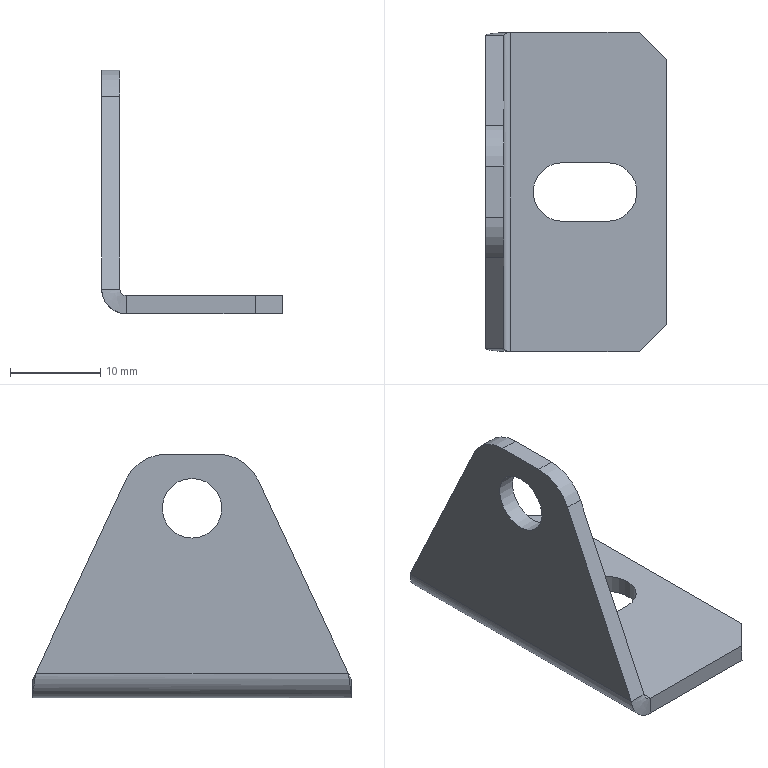Part | NX | 1 solid | 23 faces | box 20 x 35.337 x 27 mm | volume 2319 mm3 | plane 14 | cylinder 7 | spline 2 | commonest cylinder face diameters 6.5 x2 10 x2 1.473 x1 5.473 x1 6.6 x1
STEP:
#1=CARTESIAN_POINT('',(-2.5,3.25,-2.));
#2=VERTEX_POINT('',#1);
#3=CARTESIAN_POINT('',(-2.5,-3.25,-2.));
#4=VERTEX_POINT('',#3);
#5=CARTESIAN_POINT('',(-2.5,0.,-2.));
#6=DIRECTION('',(0.,0.,1.));
#7=DIRECTION('',(1.,0.,0.));
#8=AXIS2_PLACEMENT_3D('',#5,#6,#7);
#9=CIRCLE('',#8,3.25);
#10=EDGE_CURVE('',#2,#4,#9,.T.);
#11=ORIENTED_EDGE('',*,*,#10,.T.);
#12=CARTESIAN_POINT('',(2.5,-3.25,-2.));
#13=VERTEX_POINT('',#12);
#14=CARTESIAN_POINT('',(-2.5,-3.25,-2.));
#15=DIRECTION('',(1.,0.,0.));
#16=VECTOR('',#15,1000.);
#17=LINE('',#14,#16);
#18=EDGE_CURVE('',#4,#13,#17,.T.);
#19=ORIENTED_EDGE('',*,*,#18,.T.);
#20=CARTESIAN_POINT('',(2.5,3.25,-2.));
#21=VERTEX_POINT('',#20);
#22=CARTESIAN_POINT('',(2.5,0.,-2.));
#23=DIRECTION('',(0.,0.,1.));
#24=DIRECTION('',(1.,0.,0.));
#25=AXIS2_PLACEMENT_3D('',#22,#23,#24);
#26=CIRCLE('',#25,3.25);
#27=EDGE_CURVE('',#13,#21,#26,.T.);
#28=ORIENTED_EDGE('',*,*,#27,.T.);
#29=CARTESIAN_POINT('',(-2.5,3.25,-2.));
#30=DIRECTION('',(-1.,0.,0.));
#31=VECTOR('',#30,1000.);
#32=LINE('',#29,#31);
#33=EDGE_CURVE('',#21,#2,#32,.T.);
#34=ORIENTED_EDGE('',*,*,#33,.T.);
#35=EDGE_LOOP('',(#11,#19,#28,#34));
#36=FACE_BOUND('',#35,.T.);
#37=CARTESIAN_POINT('',(9.,-14.667,-2.));
#38=VERTEX_POINT('',#37);
#39=CARTESIAN_POINT('',(9.,14.67,-2.));
#40=VERTEX_POINT('',#39);
#41=CARTESIAN_POINT('',(9.,-20.,-2.));
#42=DIRECTION('',(0.,1.,0.));
#43=VECTOR('',#42,1000.);
#44=LINE('',#41,#43);
#45=EDGE_CURVE('',#38,#40,#44,.T.);
#46=ORIENTED_EDGE('',*,*,#45,.F.);
#47=CARTESIAN_POINT('',(6.,-17.667,-2.));
#48=VERTEX_POINT('',#47);
#49=CARTESIAN_POINT('',(11.833,-11.833,-2.));
#50=DIRECTION('',(0.7071,0.7071,0.));
#51=VECTOR('',#50,1000.);
#52=LINE('',#49,#51);
#53=EDGE_CURVE('',#38,#48,#52,.F.);
#54=ORIENTED_EDGE('',*,*,#53,.T.);
#55=CARTESIAN_POINT('',(-8.263,-17.667,-2.));
#56=VERTEX_POINT('',#55);
#57=CARTESIAN_POINT('',(0.,-17.667,-2.));
#58=DIRECTION('',(-1.,0.,0.));
#59=VECTOR('',#58,1000.);
#60=LINE('',#57,#59);
#61=EDGE_CURVE('',#48,#56,#60,.T.);
#62=ORIENTED_EDGE('',*,*,#61,.T.);
#63=CARTESIAN_POINT('',(-8.263,17.67,-2.));
#64=VERTEX_POINT('',#63);
#65=CARTESIAN_POINT('',(-8.263,-20.,-2.));
#66=DIRECTION('',(0.,-1.,0.));
#67=VECTOR('',#66,1000.);
#68=LINE('',#65,#67);
#69=EDGE_CURVE('',#56,#64,#68,.F.);
#70=ORIENTED_EDGE('',*,*,#69,.T.);
#71=CARTESIAN_POINT('',(6.,17.67,-2.));
#72=VERTEX_POINT('',#71);
#73=CARTESIAN_POINT('',(0.,17.67,-2.));
#74=DIRECTION('',(-1.,0.,0.));
#75=VECTOR('',#74,1000.);
#76=LINE('',#73,#75);
#77=EDGE_CURVE('',#64,#72,#76,.F.);
#78=ORIENTED_EDGE('',*,*,#77,.T.);
#79=CARTESIAN_POINT('',(11.835,11.835,-2.));
#80=DIRECTION('',(-0.7071,0.7071,0.));
#81=VECTOR('',#80,1000.);
#82=LINE('',#79,#81);
#83=EDGE_CURVE('',#72,#40,#82,.F.);
#84=ORIENTED_EDGE('',*,*,#83,.T.);
#85=EDGE_LOOP('',(#46,#54,#62,#70,#78,#84));
#86=FACE_BOUND('',#85,.T.);
#87=CARTESIAN_POINT('',(0.,0.,-2.));
#88=DIRECTION('',(0.,0.,-1.));
#89=DIRECTION('',(-1.,0.,0.));
#90=AXIS2_PLACEMENT_3D('',#87,#88,#89);
#91=PLANE('',#90);
#92=ADVANCED_FACE('',(#36,#86),#91,.T.);
#93=CARTESIAN_POINT('',(-2.5,-3.25,0.));
#94=VERTEX_POINT('',#93);
#95=CARTESIAN_POINT('',(2.5,-3.25,0.));
#96=VERTEX_POINT('',#95);
#97=CARTESIAN_POINT('',(-2.5,-3.25,0.));
#98=DIRECTION('',(1.,0.,0.));
#99=VECTOR('',#98,1000.);
#100=LINE('',#97,#99);
#101=EDGE_CURVE('',#94,#96,#100,.T.);
#102=ORIENTED_EDGE('',*,*,#101,.F.);
#103=CARTESIAN_POINT('',(-2.5,3.25,0.));
#104=VERTEX_POINT('',#103);
#105=CARTESIAN_POINT('',(-2.5,0.,0.));
#106=DIRECTION('',(0.,0.,1.));
#107=DIRECTION('',(1.,0.,0.));
#108=AXIS2_PLACEMENT_3D('',#105,#106,#107);
#109=CIRCLE('',#108,3.25);
#110=EDGE_CURVE('',#104,#94,#109,.T.);
#111=ORIENTED_EDGE('',*,*,#110,.F.);
#112=CARTESIAN_POINT('',(2.5,3.25,0.));
#113=VERTEX_POINT('',#112);
#114=CARTESIAN_POINT('',(-2.5,3.25,0.));
#115=DIRECTION('',(-1.,0.,0.));
#116=VECTOR('',#115,1000.);
#117=LINE('',#114,#116);
#118=EDGE_CURVE('',#113,#104,#117,.T.);
#119=ORIENTED_EDGE('',*,*,#118,.F.);
#120=CARTESIAN_POINT('',(2.5,0.,0.));
#121=DIRECTION('',(0.,0.,1.));
#122=DIRECTION('',(1.,0.,0.));
#123=AXIS2_PLACEMENT_3D('',#120,#121,#122);
#124=CIRCLE('',#123,3.25);
#125=EDGE_CURVE('',#96,#113,#124,.T.);
#126=ORIENTED_EDGE('',*,*,#125,.F.);
#127=EDGE_LOOP('',(#102,#111,#119,#126));
#128=FACE_BOUND('',#127,.T.);
#129=CARTESIAN_POINT('',(6.,-17.667,0.));
#130=VERTEX_POINT('',#129);
#131=CARTESIAN_POINT('',(-8.263,-17.667,0.));
#132=VERTEX_POINT('',#131);
#133=CARTESIAN_POINT('',(0.,-17.667,0.));
#134=DIRECTION('',(-1.,0.,0.));
#135=VECTOR('',#134,1000.);
#136=LINE('',#133,#135);
#137=EDGE_CURVE('',#130,#132,#136,.T.);
#138=ORIENTED_EDGE('',*,*,#137,.F.);
#139=CARTESIAN_POINT('',(9.,-14.667,0.));
#140=VERTEX_POINT('',#139);
#141=CARTESIAN_POINT('',(9.,-14.667,0.));
#142=DIRECTION('',(-0.7071,-0.7071,0.));
#143=VECTOR('',#142,1000.);
#144=LINE('',#141,#143);
#145=EDGE_CURVE('',#130,#140,#144,.F.);
#146=ORIENTED_EDGE('',*,*,#145,.T.);
#147=CARTESIAN_POINT('',(9.,14.67,0.));
#148=VERTEX_POINT('',#147);
#149=CARTESIAN_POINT('',(9.,-20.,0.));
#150=DIRECTION('',(0.,1.,0.));
#151=VECTOR('',#150,1000.);
#152=LINE('',#149,#151);
#153=EDGE_CURVE('',#140,#148,#152,.T.);
#154=ORIENTED_EDGE('',*,*,#153,.T.);
#155=CARTESIAN_POINT('',(6.,17.67,0.));
#156=VERTEX_POINT('',#155);
#157=CARTESIAN_POINT('',(6.,17.67,0.));
#158=DIRECTION('',(0.7071,-0.7071,0.));
#159=VECTOR('',#158,1000.);
#160=LINE('',#157,#159);
#161=EDGE_CURVE('',#148,#156,#160,.F.);
#162=ORIENTED_EDGE('',*,*,#161,.T.);
#163=CARTESIAN_POINT('',(-8.263,17.67,0.));
#164=VERTEX_POINT('',#163);
#165=CARTESIAN_POINT('',(0.,17.67,0.));
#166=DIRECTION('',(1.,0.,0.));
#167=VECTOR('',#166,1000.);
#168=LINE('',#165,#167);
#169=EDGE_CURVE('',#164,#156,#168,.T.);
#170=ORIENTED_EDGE('',*,*,#169,.F.);
#171=CARTESIAN_POINT('',(-8.263,-20.,0.));
#172=DIRECTION('',(0.,-1.,0.));
#173=VECTOR('',#172,1000.);
#174=LINE('',#171,#173);
#175=EDGE_CURVE('',#132,#164,#174,.F.);
#176=ORIENTED_EDGE('',*,*,#175,.F.);
#177=EDGE_LOOP('',(#138,#146,#154,#162,#170,#176));
#178=FACE_BOUND('',#177,.T.);
#179=CARTESIAN_POINT('',(0.,0.,0.));
#180=DIRECTION('',(0.,0.,-1.));
#181=DIRECTION('',(-1.,0.,0.));
#182=AXIS2_PLACEMENT_3D('',#179,#180,#181);
#183=PLANE('',#182);
#184=ADVANCED_FACE('',(#128,#178),#183,.F.);
#185=ORIENTED_EDGE('',*,*,#153,.F.);
#186=CARTESIAN_POINT('',(9.,-14.667,-2.));
#187=DIRECTION('',(0.,0.,-1.));
#188=VECTOR('',#187,1000.);
#189=LINE('',#186,#188);
#190=EDGE_CURVE('',#140,#38,#189,.T.);
#191=ORIENTED_EDGE('',*,*,#190,.T.);
#192=ORIENTED_EDGE('',*,*,#45,.T.);
#193=CARTESIAN_POINT('',(9.,14.67,-2.));
#194=DIRECTION('',(0.,0.,1.));
#195=VECTOR('',#194,1000.);
#196=LINE('',#193,#195);
#197=EDGE_CURVE('',#40,#148,#196,.T.);
#198=ORIENTED_EDGE('',*,*,#197,.T.);
#199=EDGE_LOOP('',(#185,#191,#192,#198));
#200=FACE_BOUND('',#199,.T.);
#201=CARTESIAN_POINT('',(9.,-20.,-2.));
#202=DIRECTION('',(1.,0.,0.));
#203=DIRECTION('',(0.,0.,-1.));
#204=AXIS2_PLACEMENT_3D('',#201,#202,#203);
#205=PLANE('',#204);
#206=ADVANCED_FACE('',(#200),#205,.T.);
#207=CARTESIAN_POINT('',(-11.,-17.323,0.7366));
#208=VERTEX_POINT('',#207);
#209=CARTESIAN_POINT('',(-11.,17.327,0.7366));
#210=VERTEX_POINT('',#209);
#211=CARTESIAN_POINT('',(-11.,0.,0.7366));
#212=DIRECTION('',(0.,1.,0.));
#213=VECTOR('',#212,1000.);
#214=LINE('',#211,#213);
#215=EDGE_CURVE('',#208,#210,#214,.T.);
#216=ORIENTED_EDGE('',*,*,#215,.T.);
#217=CARTESIAN_POINT('',(-8.263,17.327,0.7366));
#218=DIRECTION('',(0.,0.9922,0.1244));
#219=DIRECTION('',(0.,-0.1244,0.9922));
#220=AXIS2_PLACEMENT_3D('',#217,#218,#219);
#221=ELLIPSE('',#220,2.758,2.737);
#222=EDGE_CURVE('',#210,#64,#221,.F.);
#223=ORIENTED_EDGE('',*,*,#222,.T.);
#224=ORIENTED_EDGE('',*,*,#69,.F.);
#225=CARTESIAN_POINT('',(-8.263,-17.323,0.7366));
#226=DIRECTION('',(0.,-0.9922,0.1246));
#227=DIRECTION('',(0.,-0.1246,-0.9922));
#228=AXIS2_PLACEMENT_3D('',#225,#226,#227);
#229=ELLIPSE('',#228,2.758,2.737);
#230=EDGE_CURVE('',#56,#208,#229,.F.);
#231=ORIENTED_EDGE('',*,*,#230,.T.);
#232=EDGE_LOOP('',(#216,#223,#224,#231));
#233=FACE_BOUND('',#232,.T.);
#234=CARTESIAN_POINT('',(-8.263,-20.,0.7366));
#235=DIRECTION('',(0.,-1.,0.));
#236=DIRECTION('',(-1.,0.,0.));
#237=AXIS2_PLACEMENT_3D('',#234,#235,#236);
#238=CYLINDRICAL_SURFACE('',#237,2.737);
#239=ADVANCED_FACE('',(#233),#238,.T.);
#240=CARTESIAN_POINT('',(-9.,17.327,0.7366));
#241=VERTEX_POINT('',#240);
#242=CARTESIAN_POINT('',(-8.263,17.327,0.7366));
#243=DIRECTION('',(0.,0.9064,0.4224));
#244=DIRECTION('',(0.,-0.4224,0.9064));
#245=AXIS2_PLACEMENT_3D('',#242,#243,#244);
#246=ELLIPSE('',#245,0.8126,0.7366);
#247=EDGE_CURVE('',#241,#164,#246,.F.);
#248=ORIENTED_EDGE('',*,*,#247,.F.);
#249=CARTESIAN_POINT('',(-9.,-17.323,0.7366));
#250=VERTEX_POINT('',#249);
#251=CARTESIAN_POINT('',(-9.,20.,0.7366));
#252=DIRECTION('',(0.,-1.,0.));
#253=VECTOR('',#252,1000.);
#254=LINE('',#251,#253);
#255=EDGE_CURVE('',#241,#250,#254,.T.);
#256=ORIENTED_EDGE('',*,*,#255,.T.);
#257=CARTESIAN_POINT('',(-8.263,-17.323,0.7366));
#258=DIRECTION('',(0.,-0.9062,0.4229));
#259=DIRECTION('',(0.,-0.4229,-0.9062));
#260=AXIS2_PLACEMENT_3D('',#257,#258,#259);
#261=ELLIPSE('',#260,0.8129,0.7366);
#262=EDGE_CURVE('',#132,#250,#261,.F.);
#263=ORIENTED_EDGE('',*,*,#262,.F.);
#264=ORIENTED_EDGE('',*,*,#175,.T.);
#265=EDGE_LOOP('',(#248,#256,#263,#264));
#266=FACE_BOUND('',#265,.T.);
#267=CARTESIAN_POINT('',(-8.263,-20.,0.7366));
#268=DIRECTION('',(0.,-1.,0.));
#269=DIRECTION('',(-1.,0.,0.));
#270=AXIS2_PLACEMENT_3D('',#267,#268,#269);
#271=CYLINDRICAL_SURFACE('',#270,0.7366);
#272=ADVANCED_FACE('',(#266),#271,.F.);
#273=CARTESIAN_POINT('',(-11.,0.,22.3));
#274=VERTEX_POINT('',#273);
#275=CARTESIAN_POINT('',(-11.,0.,19.));
#276=DIRECTION('',(-1.,0.,0.));
#277=DIRECTION('',(0.,0.,1.));
#278=AXIS2_PLACEMENT_3D('',#275,#276,#277);
#279=CIRCLE('',#278,3.3);
#280=EDGE_CURVE('',#274,#274,#279,.T.);
#281=ORIENTED_EDGE('',*,*,#280,.F.);
#282=EDGE_LOOP('',(#281));
#283=FACE_BOUND('',#282,.T.);
#284=CARTESIAN_POINT('',(-11.,-2.816,25.));
#285=VERTEX_POINT('',#284);
#286=CARTESIAN_POINT('',(-11.,2.835,25.));
#287=VERTEX_POINT('',#286);
#288=CARTESIAN_POINT('',(-11.,20.,25.));
#289=DIRECTION('',(0.,1.,0.));
#290=VECTOR('',#289,1000.);
#291=LINE('',#288,#290);
#292=EDGE_CURVE('',#285,#287,#291,.T.);
#293=ORIENTED_EDGE('',*,*,#292,.T.);
#294=CARTESIAN_POINT('',(-11.,7.367,22.112));
#295=VERTEX_POINT('',#294);
#296=CARTESIAN_POINT('',(-11.,2.835,20.));
#297=DIRECTION('',(1.,0.,0.));
#298=DIRECTION('',(0.,0.,-1.));
#299=AXIS2_PLACEMENT_3D('',#296,#297,#298);
#300=CIRCLE('',#299,5.);
#301=EDGE_CURVE('',#287,#295,#300,.F.);
#302=ORIENTED_EDGE('',*,*,#301,.T.);
#303=CARTESIAN_POINT('',(-11.,14.518,6.765));
#304=DIRECTION('',(0.,-0.4224,0.9064));
#305=VECTOR('',#304,1000.);
#306=LINE('',#303,#305);
#307=EDGE_CURVE('',#210,#295,#306,.T.);
#308=ORIENTED_EDGE('',*,*,#307,.F.);
#309=ORIENTED_EDGE('',*,*,#215,.F.);
#310=CARTESIAN_POINT('',(-11.,-7.347,22.114));
#311=VERTEX_POINT('',#310);
#312=CARTESIAN_POINT('',(-11.,-6.,25.));
#313=DIRECTION('',(0.,0.4229,0.9062));
#314=VECTOR('',#313,1000.);
#315=LINE('',#312,#314);
#316=EDGE_CURVE('',#208,#311,#315,.T.);
#317=ORIENTED_EDGE('',*,*,#316,.T.);
#318=CARTESIAN_POINT('',(-11.,-2.816,20.));
#319=DIRECTION('',(1.,0.,0.));
#320=DIRECTION('',(0.,0.,-1.));
#321=AXIS2_PLACEMENT_3D('',#318,#319,#320);
#322=CIRCLE('',#321,5.);
#323=EDGE_CURVE('',#311,#285,#322,.F.);
#324=ORIENTED_EDGE('',*,*,#323,.T.);
#325=EDGE_LOOP('',(#293,#302,#308,#309,#317,#324));
#326=FACE_BOUND('',#325,.T.);
#327=CARTESIAN_POINT('',(-11.,0.,0.));
#328=DIRECTION('',(1.,0.,0.));
#329=DIRECTION('',(0.,0.,-1.));
#330=AXIS2_PLACEMENT_3D('',#327,#328,#329);
#331=PLANE('',#330);
#332=ADVANCED_FACE('',(#283,#326),#331,.F.);
#333=CARTESIAN_POINT('',(-9.,0.,15.7));
#334=VERTEX_POINT('',#333);
#335=CARTESIAN_POINT('',(-9.,0.,19.));
#336=DIRECTION('',(1.,0.,0.));
#337=DIRECTION('',(0.,0.,-1.));
#338=AXIS2_PLACEMENT_3D('',#335,#336,#337);
#339=CIRCLE('',#338,3.3);
#340=EDGE_CURVE('',#334,#334,#339,.T.);
#341=ORIENTED_EDGE('',*,*,#340,.F.);
#342=EDGE_LOOP('',(#341));
#343=FACE_BOUND('',#342,.T.);
#344=CARTESIAN_POINT('',(-9.,7.367,22.112));
#345=VERTEX_POINT('',#344);
#346=CARTESIAN_POINT('',(-9.,14.518,6.765));
#347=DIRECTION('',(0.,-0.4224,0.9064));
#348=VECTOR('',#347,1000.);
#349=LINE('',#346,#348);
#350=EDGE_CURVE('',#241,#345,#349,.T.);
#351=ORIENTED_EDGE('',*,*,#350,.T.);
#352=CARTESIAN_POINT('',(-9.,2.835,25.));
#353=VERTEX_POINT('',#352);
#354=CARTESIAN_POINT('',(-9.,2.835,20.));
#355=DIRECTION('',(1.,0.,0.));
#356=DIRECTION('',(0.,0.,-1.));
#357=AXIS2_PLACEMENT_3D('',#354,#355,#356);
#358=CIRCLE('',#357,5.);
#359=EDGE_CURVE('',#345,#353,#358,.T.);
#360=ORIENTED_EDGE('',*,*,#359,.T.);
#361=CARTESIAN_POINT('',(-9.,-2.816,25.));
#362=VERTEX_POINT('',#361);
#363=CARTESIAN_POINT('',(-9.,20.,25.));
#364=DIRECTION('',(0.,1.,0.));
#365=VECTOR('',#364,1000.);
#366=LINE('',#363,#365);
#367=EDGE_CURVE('',#362,#353,#366,.T.);
#368=ORIENTED_EDGE('',*,*,#367,.F.);
#369=CARTESIAN_POINT('',(-9.,-7.347,22.114));
#370=VERTEX_POINT('',#369);
#371=CARTESIAN_POINT('',(-9.,-2.816,20.));
#372=DIRECTION('',(1.,0.,0.));
#373=DIRECTION('',(0.,0.,-1.));
#374=AXIS2_PLACEMENT_3D('',#371,#372,#373);
#375=CIRCLE('',#374,5.);
#376=EDGE_CURVE('',#362,#370,#375,.T.);
#377=ORIENTED_EDGE('',*,*,#376,.T.);
#378=CARTESIAN_POINT('',(-9.,-6.,25.));
#379=DIRECTION('',(0.,0.4229,0.9062));
#380=VECTOR('',#379,1000.);
#381=LINE('',#378,#380);
#382=EDGE_CURVE('',#250,#370,#381,.T.);
#383=ORIENTED_EDGE('',*,*,#382,.F.);
#384=ORIENTED_EDGE('',*,*,#255,.F.);
#385=EDGE_LOOP('',(#351,#360,#368,#377,#383,#384));
#386=FACE_BOUND('',#385,.T.);
#387=CARTESIAN_POINT('',(-9.,0.,0.));
#388=DIRECTION('',(1.,0.,0.));
#389=DIRECTION('',(0.,0.,-1.));
#390=AXIS2_PLACEMENT_3D('',#387,#388,#389);
#391=PLANE('',#390);
#392=ADVANCED_FACE('',(#343,#386),#391,.T.);
#393=ORIENTED_EDGE('',*,*,#367,.T.);
#394=CARTESIAN_POINT('',(-11.,2.835,25.));
#395=DIRECTION('',(-1.,0.,0.));
#396=VECTOR('',#395,1000.);
#397=LINE('',#394,#396);
#398=EDGE_CURVE('',#353,#287,#397,.T.);
#399=ORIENTED_EDGE('',*,*,#398,.T.);
#400=ORIENTED_EDGE('',*,*,#292,.F.);
#401=CARTESIAN_POINT('',(-9.,-2.816,25.));
#402=DIRECTION('',(-1.,0.,0.));
#403=VECTOR('',#402,1000.);
#404=LINE('',#401,#403);
#405=EDGE_CURVE('',#285,#362,#404,.F.);
#406=ORIENTED_EDGE('',*,*,#405,.T.);
#407=EDGE_LOOP('',(#393,#399,#400,#406));
#408=FACE_BOUND('',#407,.T.);
#409=CARTESIAN_POINT('',(-11.,20.,25.));
#410=DIRECTION('',(0.,0.,-1.));
#411=DIRECTION('',(-1.,0.,0.));
#412=AXIS2_PLACEMENT_3D('',#409,#410,#411);
#413=PLANE('',#412);
#414=ADVANCED_FACE('',(#408),#413,.F.);
#415=ORIENTED_EDGE('',*,*,#61,.F.);
#416=CARTESIAN_POINT('',(6.,-17.667,0.));
#417=DIRECTION('',(0.,0.,1.));
#418=VECTOR('',#417,1000.);
#419=LINE('',#416,#418);
#420=EDGE_CURVE('',#48,#130,#419,.T.);
#421=ORIENTED_EDGE('',*,*,#420,.T.);
#422=ORIENTED_EDGE('',*,*,#137,.T.);
#423=CARTESIAN_POINT('',(-8.263,-17.667,0.));
#424=DIRECTION('',(0.,0.,1.));
#425=VECTOR('',#424,1000.);
#426=LINE('',#423,#425);
#427=EDGE_CURVE('',#132,#56,#426,.F.);
#428=ORIENTED_EDGE('',*,*,#427,.T.);
#429=EDGE_LOOP('',(#415,#421,#422,#428));
#430=FACE_BOUND('',#429,.T.);
#431=CARTESIAN_POINT('',(0.,-17.667,0.));
#432=DIRECTION('',(0.,-1.,0.));
#433=DIRECTION('',(-1.,0.,0.));
#434=AXIS2_PLACEMENT_3D('',#431,#432,#433);
#435=PLANE('',#434);
#436=ADVANCED_FACE('',(#430),#435,.T.);
#437=ORIENTED_EDGE('',*,*,#382,.T.);
#438=CARTESIAN_POINT('',(-11.,-7.347,22.114));
#439=DIRECTION('',(1.,0.,0.));
#440=VECTOR('',#439,1000.);
#441=LINE('',#438,#440);
#442=EDGE_CURVE('',#370,#311,#441,.F.);
#443=ORIENTED_EDGE('',*,*,#442,.T.);
#444=ORIENTED_EDGE('',*,*,#316,.F.);
#445=CARTESIAN_POINT('',(-11.,-17.323,0.7366));
#446=DIRECTION('',(-1.,0.,0.));
#447=VECTOR('',#446,1000.);
#448=LINE('',#445,#447);
#449=EDGE_CURVE('',#208,#250,#448,.F.);
#450=ORIENTED_EDGE('',*,*,#449,.T.);
#451=EDGE_LOOP('',(#437,#443,#444,#450));
#452=FACE_BOUND('',#451,.T.);
#453=CARTESIAN_POINT('',(-11.,-6.,25.));
#454=DIRECTION('',(0.,0.9062,-0.4229));
#455=DIRECTION('',(0.,0.4229,0.9062));
#456=AXIS2_PLACEMENT_3D('',#453,#454,#455);
#457=PLANE('',#456);
#458=ADVANCED_FACE('',(#452),#457,.F.);
#459=ORIENTED_EDGE('',*,*,#262,.T.);
#460=ORIENTED_EDGE('',*,*,#449,.F.);
#461=ORIENTED_EDGE('',*,*,#230,.F.);
#462=ORIENTED_EDGE('',*,*,#427,.F.);
#463=EDGE_LOOP('',(#459,#460,#461,#462));
#464=FACE_BOUND('',#463,.T.);
#465=CARTESIAN_POINT('',(-8.263,-17.667,-2.));
#466=CARTESIAN_POINT('',(-8.263,-17.667,-1.333));
#467=CARTESIAN_POINT('',(-8.263,-17.667,-0.6667));
#468=CARTESIAN_POINT('',(-8.263,-17.667,0.));
#469=CARTESIAN_POINT('',(-9.632,-17.667,-2.));
#470=CARTESIAN_POINT('',(-9.298,-17.667,-1.333));
#471=CARTESIAN_POINT('',(-8.965,-17.667,-0.6667));
#472=CARTESIAN_POINT('',(-8.632,-17.667,0.));
#473=CARTESIAN_POINT('',(-11.,-17.552,-1.088));
#474=CARTESIAN_POINT('',(-10.333,-17.552,-0.6434));
#475=CARTESIAN_POINT('',(-9.667,-17.552,-0.1989));
#476=CARTESIAN_POINT('',(-9.,-17.552,0.2455));
#477=CARTESIAN_POINT('',(-11.,-17.323,0.7366));
#478=CARTESIAN_POINT('',(-10.333,-17.323,0.7366));
#479=CARTESIAN_POINT('',(-9.667,-17.323,0.7366));
#480=CARTESIAN_POINT('',(-9.,-17.323,0.7366));
#481=(BOUNDED_SURFACE()B_SPLINE_SURFACE(3,3,((#465,#466,#467,#468),(#469,#470,#471,#472),(#473,#474,#475,#476),(#477,#478,#479,#480)),.RULED_SURF.,.F.,.F.,.F.)B_SPLINE_SURFACE_WITH_KNOTS((4,4),(4,4),(0.,0.25),(0.,1.),.PIECEWISE_BEZIER_KNOTS.)GEOMETRIC_REPRESENTATION_ITEM()RATIONAL_B_SPLINE_SURFACE(((1.,1.,1.,1.),(0.6667,0.6667,0.6667,0.6667),(0.5,0.5,0.5,0.5),(0.5,0.5,0.5,0.5)))REPRESENTATION_ITEM('')SURFACE());
#482=ADVANCED_FACE('',(#464),#481,.F.);
#483=ORIENTED_EDGE('',*,*,#169,.T.);
#484=CARTESIAN_POINT('',(6.,17.67,0.));
#485=DIRECTION('',(0.,0.,-1.));
#486=VECTOR('',#485,1000.);
#487=LINE('',#484,#486);
#488=EDGE_CURVE('',#156,#72,#487,.T.);
#489=ORIENTED_EDGE('',*,*,#488,.T.);
#490=ORIENTED_EDGE('',*,*,#77,.F.);
#491=CARTESIAN_POINT('',(-8.263,17.67,0.));
#492=DIRECTION('',(0.,0.,1.));
#493=VECTOR('',#492,1000.);
#494=LINE('',#491,#493);
#495=EDGE_CURVE('',#164,#64,#494,.F.);
#496=ORIENTED_EDGE('',*,*,#495,.F.);
#497=EDGE_LOOP('',(#483,#489,#490,#496));
#498=FACE_BOUND('',#497,.T.);
#499=CARTESIAN_POINT('',(0.,17.67,0.));
#500=DIRECTION('',(0.,1.,0.));
#501=DIRECTION('',(1.,0.,0.));
#502=AXIS2_PLACEMENT_3D('',#499,#500,#501);
#503=PLANE('',#502);
#504=ADVANCED_FACE('',(#498),#503,.T.);
#505=ORIENTED_EDGE('',*,*,#307,.T.);
#506=CARTESIAN_POINT('',(-9.,7.367,22.112));
#507=DIRECTION('',(-1.,0.,0.));
#508=VECTOR('',#507,1000.);
#509=LINE('',#506,#508);
#510=EDGE_CURVE('',#295,#345,#509,.F.);
#511=ORIENTED_EDGE('',*,*,#510,.T.);
#512=ORIENTED_EDGE('',*,*,#350,.F.);
#513=CARTESIAN_POINT('',(-9.,17.327,0.7366));
#514=DIRECTION('',(1.,0.,0.));
#515=VECTOR('',#514,1000.);
#516=LINE('',#513,#515);
#517=EDGE_CURVE('',#241,#210,#516,.F.);
#518=ORIENTED_EDGE('',*,*,#517,.T.);
#519=EDGE_LOOP('',(#505,#511,#512,#518));
#520=FACE_BOUND('',#519,.T.);
#521=CARTESIAN_POINT('',(-9.,14.518,6.765));
#522=DIRECTION('',(0.,0.9064,0.4224));
#523=DIRECTION('',(0.,-0.4224,0.9064));
#524=AXIS2_PLACEMENT_3D('',#521,#522,#523);
#525=PLANE('',#524);
#526=ADVANCED_FACE('',(#520),#525,.T.);
#527=ORIENTED_EDGE('',*,*,#247,.T.);
#528=ORIENTED_EDGE('',*,*,#495,.T.);
#529=ORIENTED_EDGE('',*,*,#222,.F.);
#530=ORIENTED_EDGE('',*,*,#517,.F.);
#531=EDGE_LOOP('',(#527,#528,#529,#530));
#532=FACE_BOUND('',#531,.T.);
#533=CARTESIAN_POINT('',(-11.,17.327,0.7366));
#534=CARTESIAN_POINT('',(-10.333,17.327,0.7366));
#535=CARTESIAN_POINT('',(-9.667,17.327,0.7366));
#536=CARTESIAN_POINT('',(-9.,17.327,0.7366));
#537=CARTESIAN_POINT('',(-11.,17.556,-1.088));
#538=CARTESIAN_POINT('',(-10.333,17.556,-0.6434));
#539=CARTESIAN_POINT('',(-9.667,17.556,-0.1989));
#540=CARTESIAN_POINT('',(-9.,17.556,0.2455));
#541=CARTESIAN_POINT('',(-9.632,17.67,-2.));
#542=CARTESIAN_POINT('',(-9.298,17.67,-1.333));
#543=CARTESIAN_POINT('',(-8.965,17.67,-0.6667));
#544=CARTESIAN_POINT('',(-8.632,17.67,0.));
#545=CARTESIAN_POINT('',(-8.263,17.67,-2.));
#546=CARTESIAN_POINT('',(-8.263,17.67,-1.333));
#547=CARTESIAN_POINT('',(-8.263,17.67,-0.6667));
#548=CARTESIAN_POINT('',(-8.263,17.67,0.));
#549=(BOUNDED_SURFACE()B_SPLINE_SURFACE(3,3,((#533,#534,#535,#536),(#537,#538,#539,#540),(#541,#542,#543,#544),(#545,#546,#547,#548)),.RULED_SURF.,.F.,.F.,.F.)B_SPLINE_SURFACE_WITH_KNOTS((4,4),(4,4),(0.25,0.5),(0.,1.),.PIECEWISE_BEZIER_KNOTS.)GEOMETRIC_REPRESENTATION_ITEM()RATIONAL_B_SPLINE_SURFACE(((0.5,0.5,0.5,0.5),(0.5,0.5,0.5,0.5),(0.6667,0.6667,0.6667,0.6667),(1.,1.,1.,1.)))REPRESENTATION_ITEM('')SURFACE());
#550=ADVANCED_FACE('',(#532),#549,.F.);
#551=ORIENTED_EDGE('',*,*,#359,.F.);
#552=ORIENTED_EDGE('',*,*,#510,.F.);
#553=ORIENTED_EDGE('',*,*,#301,.F.);
#554=ORIENTED_EDGE('',*,*,#398,.F.);
#555=EDGE_LOOP('',(#551,#552,#553,#554));
#556=FACE_BOUND('',#555,.T.);
#557=CARTESIAN_POINT('',(-11.,2.835,20.));
#558=DIRECTION('',(1.,0.,0.));
#559=DIRECTION('',(0.,0.,-1.));
#560=AXIS2_PLACEMENT_3D('',#557,#558,#559);
#561=CYLINDRICAL_SURFACE('',#560,5.);
#562=ADVANCED_FACE('',(#556),#561,.T.);
#563=ORIENTED_EDGE('',*,*,#323,.F.);
#564=ORIENTED_EDGE('',*,*,#442,.F.);
#565=ORIENTED_EDGE('',*,*,#376,.F.);
#566=ORIENTED_EDGE('',*,*,#405,.F.);
#567=EDGE_LOOP('',(#563,#564,#565,#566));
#568=FACE_BOUND('',#567,.T.);
#569=CARTESIAN_POINT('',(-11.,-2.816,20.));
#570=DIRECTION('',(1.,0.,0.));
#571=DIRECTION('',(0.,0.,-1.));
#572=AXIS2_PLACEMENT_3D('',#569,#570,#571);
#573=CYLINDRICAL_SURFACE('',#572,5.);
#574=ADVANCED_FACE('',(#568),#573,.T.);
#575=ORIENTED_EDGE('',*,*,#340,.T.);
#576=EDGE_LOOP('',(#575));
#577=FACE_BOUND('',#576,.T.);
#578=ORIENTED_EDGE('',*,*,#280,.T.);
#579=EDGE_LOOP('',(#578));
#580=FACE_BOUND('',#579,.T.);
#581=CARTESIAN_POINT('',(-11.,0.,19.));
#582=DIRECTION('',(-1.,0.,0.));
#583=DIRECTION('',(0.,0.,1.));
#584=AXIS2_PLACEMENT_3D('',#581,#582,#583);
#585=CYLINDRICAL_SURFACE('',#584,3.3);
#586=ADVANCED_FACE('',(#577,#580),#585,.F.);
#587=ORIENTED_EDGE('',*,*,#110,.T.);
#588=CARTESIAN_POINT('',(-2.5,-3.25,-2.));
#589=DIRECTION('',(0.,0.,1.));
#590=VECTOR('',#589,1000.);
#591=LINE('',#588,#590);
#592=EDGE_CURVE('',#4,#94,#591,.T.);
#593=ORIENTED_EDGE('',*,*,#592,.F.);
#594=ORIENTED_EDGE('',*,*,#10,.F.);
#595=CARTESIAN_POINT('',(-2.5,3.25,-2.));
#596=DIRECTION('',(0.,0.,1.));
#597=VECTOR('',#596,1000.);
#598=LINE('',#595,#597);
#599=EDGE_CURVE('',#2,#104,#598,.T.);
#600=ORIENTED_EDGE('',*,*,#599,.T.);
#601=EDGE_LOOP('',(#587,#593,#594,#600));
#602=FACE_BOUND('',#601,.T.);
#603=CARTESIAN_POINT('',(-2.5,0.,-2.));
#604=DIRECTION('',(0.,0.,1.));
#605=DIRECTION('',(1.,0.,0.));
#606=AXIS2_PLACEMENT_3D('',#603,#604,#605);
#607=CYLINDRICAL_SURFACE('',#606,3.25);
#608=ADVANCED_FACE('',(#602),#607,.F.);
#609=ORIENTED_EDGE('',*,*,#118,.T.);
#610=ORIENTED_EDGE('',*,*,#599,.F.);
#611=ORIENTED_EDGE('',*,*,#33,.F.);
#612=CARTESIAN_POINT('',(2.5,3.25,-2.));
#613=DIRECTION('',(0.,0.,1.));
#614=VECTOR('',#613,1000.);
#615=LINE('',#612,#614);
#616=EDGE_CURVE('',#21,#113,#615,.T.);
#617=ORIENTED_EDGE('',*,*,#616,.T.);
#618=EDGE_LOOP('',(#609,#610,#611,#617));
#619=FACE_BOUND('',#618,.T.);
#620=CARTESIAN_POINT('',(-2.5,3.25,-2.));
#621=DIRECTION('',(0.,1.,0.));
#622=DIRECTION('',(-1.,0.,0.));
#623=AXIS2_PLACEMENT_3D('',#620,#621,#622);
#624=PLANE('',#623);
#625=ADVANCED_FACE('',(#619),#624,.F.);
#626=ORIENTED_EDGE('',*,*,#125,.T.);
#627=ORIENTED_EDGE('',*,*,#616,.F.);
#628=ORIENTED_EDGE('',*,*,#27,.F.);
#629=CARTESIAN_POINT('',(2.5,-3.25,-2.));
#630=DIRECTION('',(0.,0.,1.));
#631=VECTOR('',#630,1000.);
#632=LINE('',#629,#631);
#633=EDGE_CURVE('',#13,#96,#632,.T.);
#634=ORIENTED_EDGE('',*,*,#633,.T.);
#635=EDGE_LOOP('',(#626,#627,#628,#634));
#636=FACE_BOUND('',#635,.T.);
#637=CARTESIAN_POINT('',(2.5,0.,-2.));
#638=DIRECTION('',(0.,0.,1.));
#639=DIRECTION('',(1.,0.,0.));
#640=AXIS2_PLACEMENT_3D('',#637,#638,#639);
#641=CYLINDRICAL_SURFACE('',#640,3.25);
#642=ADVANCED_FACE('',(#636),#641,.F.);
#643=ORIENTED_EDGE('',*,*,#101,.T.);
#644=ORIENTED_EDGE('',*,*,#633,.F.);
#645=ORIENTED_EDGE('',*,*,#18,.F.);
#646=ORIENTED_EDGE('',*,*,#592,.T.);
#647=EDGE_LOOP('',(#643,#644,#645,#646));
#648=FACE_BOUND('',#647,.T.);
#649=CARTESIAN_POINT('',(-2.5,-3.25,-2.));
#650=DIRECTION('',(0.,-1.,0.));
#651=DIRECTION('',(1.,0.,0.));
#652=AXIS2_PLACEMENT_3D('',#649,#650,#651);
#653=PLANE('',#652);
#654=ADVANCED_FACE('',(#648),#653,.F.);
#655=ORIENTED_EDGE('',*,*,#145,.F.);
#656=ORIENTED_EDGE('',*,*,#420,.F.);
#657=ORIENTED_EDGE('',*,*,#53,.F.);
#658=ORIENTED_EDGE('',*,*,#190,.F.);
#659=EDGE_LOOP('',(#655,#656,#657,#658));
#660=FACE_BOUND('',#659,.T.);
#661=CARTESIAN_POINT('',(9.,-14.667,-2.));
#662=DIRECTION('',(-0.7071,0.7071,0.));
#663=DIRECTION('',(0.,0.,-1.));
#664=AXIS2_PLACEMENT_3D('',#661,#662,#663);
#665=PLANE('',#664);
#666=ADVANCED_FACE('',(#660),#665,.F.);
#667=ORIENTED_EDGE('',*,*,#161,.F.);
#668=ORIENTED_EDGE('',*,*,#197,.F.);
#669=ORIENTED_EDGE('',*,*,#83,.F.);
#670=ORIENTED_EDGE('',*,*,#488,.F.);
#671=EDGE_LOOP('',(#667,#668,#669,#670));
#672=FACE_BOUND('',#671,.T.);
#673=CARTESIAN_POINT('',(6.,17.67,0.));
#674=DIRECTION('',(-0.7071,-0.7071,0.));
#675=DIRECTION('',(0.,0.,-1.));
#676=AXIS2_PLACEMENT_3D('',#673,#674,#675);
#677=PLANE('',#676);
#678=ADVANCED_FACE('',(#672),#677,.F.);
#679=CLOSED_SHELL('',(#92,#184,#206,#239,#272,#332,#392,#414,#436,#458,#482,#504,#526,#550,#562,#574,#586,#608,#625,#642,#654,#666,#678));
#680=MANIFOLD_SOLID_BREP('',#679);
#681=(LENGTH_UNIT()NAMED_UNIT(*)SI_UNIT(.MILLI.,.METRE.));
#682=UNCERTAINTY_MEASURE_WITH_UNIT(LENGTH_MEASURE(0.00001),#681,'','');
#683=(NAMED_UNIT(*)PLANE_ANGLE_UNIT()SI_UNIT($,.RADIAN.));
#684=(NAMED_UNIT(*)SI_UNIT($,.STERADIAN.)SOLID_ANGLE_UNIT());
#685=(GEOMETRIC_REPRESENTATION_CONTEXT(3)GLOBAL_UNCERTAINTY_ASSIGNED_CONTEXT((#682))GLOBAL_UNIT_ASSIGNED_CONTEXT((#681,#683,#684))REPRESENTATION_CONTEXT('',''));
#686=ADVANCED_BREP_SHAPE_REPRESENTATION('',(#680),#685);